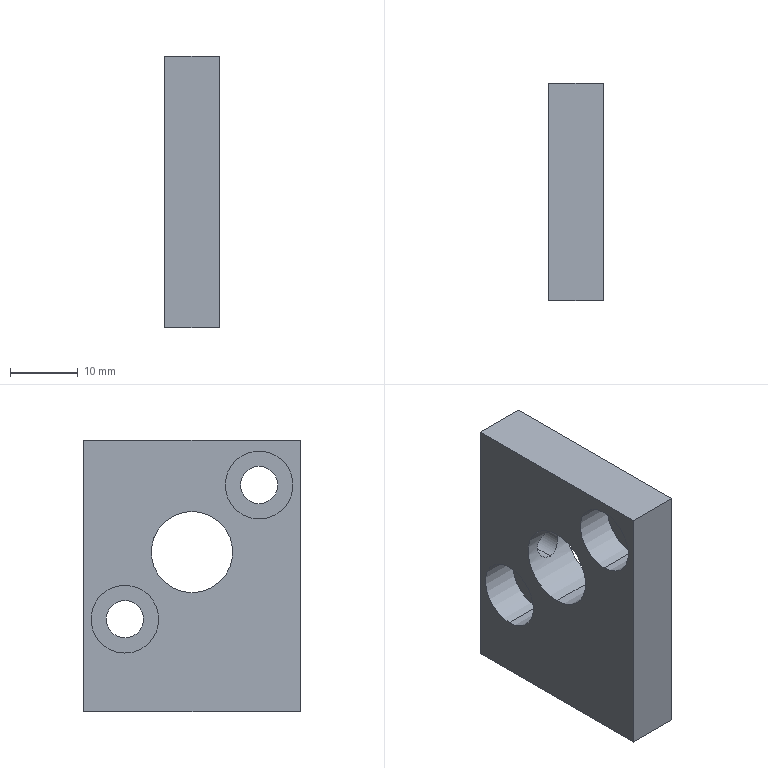Part | SolidWorks | features HoleWzd 2, Extrusion 1, ICE 1 | 1 solid | 28 faces | box 8 x 32 x 40 mm | volume 7835 mm3 | cylinder 16 | plane 8 | cone 4 | commonest cylinder face diameters 4.2 x6 5.5 x4 10 x4 12 x2
STEP:
#1=CARTESIAN_POINT('',(4.,5.396,0.9));
#2=VERTEX_POINT('',#1);
#3=CARTESIAN_POINT('',(4.,5.789,5.1));
#4=VERTEX_POINT('',#3);
#5=CARTESIAN_POINT('',(4.,5.396,0.9));
#6=CARTESIAN_POINT('',(3.724,5.396,0.9));
#7=CARTESIAN_POINT('',(3.445,5.424,0.9562));
#8=CARTESIAN_POINT('',(3.067,5.495,1.114));
#9=CARTESIAN_POINT('',(2.945,5.524,1.179));
#10=CARTESIAN_POINT('',(2.72,5.585,1.33));
#11=CARTESIAN_POINT('',(2.616,5.618,1.415));
#12=CARTESIAN_POINT('',(2.423,5.686,1.606));
#13=CARTESIAN_POINT('',(2.337,5.721,1.71));
#14=CARTESIAN_POINT('',(2.187,5.786,1.932));
#15=CARTESIAN_POINT('',(2.121,5.818,2.052));
#16=CARTESIAN_POINT('',(2.014,5.876,2.303));
#17=CARTESIAN_POINT('',(1.974,5.901,2.432));
#18=CARTESIAN_POINT('',(1.917,5.945,2.699));
#19=CARTESIAN_POINT('',(1.902,5.962,2.839));
#20=CARTESIAN_POINT('',(1.899,5.988,3.115));
#21=CARTESIAN_POINT('',(1.911,5.995,3.252));
#22=CARTESIAN_POINT('',(1.962,6.002,3.525));
#23=CARTESIAN_POINT('',(2.002,6.,3.661));
#24=CARTESIAN_POINT('',(2.158,5.983,4.045));
#25=CARTESIAN_POINT('',(2.314,5.955,4.282));
#26=CARTESIAN_POINT('',(2.604,5.908,4.575));
#27=CARTESIAN_POINT('',(2.712,5.891,4.665));
#28=CARTESIAN_POINT('',(2.941,5.859,4.819));
#29=CARTESIAN_POINT('',(3.062,5.844,4.884));
#30=CARTESIAN_POINT('',(3.318,5.818,4.991));
#31=CARTESIAN_POINT('',(3.452,5.807,5.032));
#32=CARTESIAN_POINT('',(3.722,5.793,5.086));
#33=CARTESIAN_POINT('',(3.86,5.789,5.1));
#34=CARTESIAN_POINT('',(4.,5.789,5.1));
#35=B_SPLINE_CURVE_WITH_KNOTS('',3,(#5,#6,#7,#8,#9,#10,#11,#12,#13,#14,#15,#16,#17,#18,#19,#20,#21,#22,#23,#24,#25,#26,#27,#28,#29,#30,#31,#32,#33,#34),.UNSPECIFIED.,.F.,.F.,(4,2,2,2,2,2,2,2,2,2,2,2,2,2,4),(0.006634,0.007462,0.007877,0.008291,0.008706,0.00912,0.009534,0.009949,0.01036,0.01078,0.01161,0.01202,0.01243,0.01285,0.01326),.UNSPECIFIED.);
#36=EDGE_CURVE('',#2,#4,#35,.T.);
#37=ORIENTED_EDGE('',*,*,#36,.F.);
#38=CARTESIAN_POINT('',(4.,16.,0.9));
#39=VERTEX_POINT('',#38);
#40=CARTESIAN_POINT('',(4.,16.,0.9));
#41=DIRECTION('',(0.,1.,0.));
#42=VECTOR('',#41,1000.);
#43=LINE('',#40,#42);
#44=EDGE_CURVE('',#2,#39,#43,.T.);
#45=ORIENTED_EDGE('',*,*,#44,.T.);
#46=CARTESIAN_POINT('',(4.,16.,5.1));
#47=VERTEX_POINT('',#46);
#48=CARTESIAN_POINT('',(4.,16.,3.));
#49=DIRECTION('',(0.,1.,0.));
#50=DIRECTION('',(0.,0.,1.));
#51=AXIS2_PLACEMENT_3D('',#48,#49,#50);
#52=CIRCLE('',#51,2.1);
#53=EDGE_CURVE('',#39,#47,#52,.T.);
#54=ORIENTED_EDGE('',*,*,#53,.T.);
#55=CARTESIAN_POINT('',(4.,16.,5.1));
#56=DIRECTION('',(0.,1.,0.));
#57=VECTOR('',#56,1000.);
#58=LINE('',#55,#57);
#59=EDGE_CURVE('',#4,#47,#58,.T.);
#60=ORIENTED_EDGE('',*,*,#59,.F.);
#61=EDGE_LOOP('',(#37,#45,#54,#60));
#62=FACE_OUTER_BOUND('',#61,.T.);
#63=CARTESIAN_POINT('',(4.,16.,3.));
#64=DIRECTION('',(0.,1.,0.));
#65=DIRECTION('',(0.,0.,1.));
#66=AXIS2_PLACEMENT_3D('',#63,#64,#65);
#67=CYLINDRICAL_SURFACE('',#66,2.1);
#68=ADVANCED_FACE('',(#62),#67,.F.);
#69=CARTESIAN_POINT('',(4.,3.6,12.9));
#70=VERTEX_POINT('',#69);
#71=CARTESIAN_POINT('',(4.,3.6,17.1));
#72=VERTEX_POINT('',#71);
#73=CARTESIAN_POINT('',(4.,3.6,15.));
#74=DIRECTION('',(0.,1.,0.));
#75=DIRECTION('',(0.,0.,1.));
#76=AXIS2_PLACEMENT_3D('',#73,#74,#75);
#77=CIRCLE('',#76,2.1);
#78=EDGE_CURVE('',#70,#72,#77,.T.);
#79=ORIENTED_EDGE('',*,*,#78,.F.);
#80=CARTESIAN_POINT('',(4.,16.,12.9));
#81=VERTEX_POINT('',#80);
#82=CARTESIAN_POINT('',(4.,16.,12.9));
#83=DIRECTION('',(0.,1.,0.));
#84=VECTOR('',#83,1000.);
#85=LINE('',#82,#84);
#86=EDGE_CURVE('',#70,#81,#85,.T.);
#87=ORIENTED_EDGE('',*,*,#86,.T.);
#88=CARTESIAN_POINT('',(4.,16.,17.1));
#89=VERTEX_POINT('',#88);
#90=CARTESIAN_POINT('',(4.,16.,15.));
#91=DIRECTION('',(0.,1.,0.));
#92=DIRECTION('',(0.,0.,1.));
#93=AXIS2_PLACEMENT_3D('',#90,#91,#92);
#94=CIRCLE('',#93,2.1);
#95=EDGE_CURVE('',#81,#89,#94,.T.);
#96=ORIENTED_EDGE('',*,*,#95,.T.);
#97=CARTESIAN_POINT('',(4.,16.,17.1));
#98=DIRECTION('',(0.,1.,0.));
#99=VECTOR('',#98,1000.);
#100=LINE('',#97,#99);
#101=EDGE_CURVE('',#72,#89,#100,.T.);
#102=ORIENTED_EDGE('',*,*,#101,.F.);
#103=EDGE_LOOP('',(#79,#87,#96,#102));
#104=FACE_OUTER_BOUND('',#103,.T.);
#105=CARTESIAN_POINT('',(4.,16.,15.));
#106=DIRECTION('',(0.,1.,0.));
#107=DIRECTION('',(0.,0.,1.));
#108=AXIS2_PLACEMENT_3D('',#105,#106,#107);
#109=CYLINDRICAL_SURFACE('',#108,2.1);
#110=ADVANCED_FACE('',(#104),#109,.F.);
#111=CARTESIAN_POINT('',(4.,2.338,15.));
#112=VERTEX_POINT('',#111);
#113=CARTESIAN_POINT('',(4.,3.6,17.1));
#114=DIRECTION('',(0.,0.515,0.8572));
#115=VECTOR('',#114,1000.);
#116=LINE('',#113,#115);
#117=EDGE_CURVE('',#112,#72,#116,.T.);
#118=ORIENTED_EDGE('',*,*,#117,.F.);
#119=CARTESIAN_POINT('',(4.,3.6,12.9));
#120=DIRECTION('',(0.,0.515,-0.8572));
#121=VECTOR('',#120,1000.);
#122=LINE('',#119,#121);
#123=EDGE_CURVE('',#112,#70,#122,.T.);
#124=ORIENTED_EDGE('',*,*,#123,.T.);
#125=ORIENTED_EDGE('',*,*,#78,.T.);
#126=EDGE_LOOP('',(#118,#124,#125));
#127=FACE_OUTER_BOUND('',#126,.T.);
#128=CARTESIAN_POINT('',(4.,3.6,15.));
#129=DIRECTION('',(0.,1.,0.));
#130=DIRECTION('',(0.,0.,1.));
#131=AXIS2_PLACEMENT_3D('',#128,#129,#130);
#132=CONICAL_SURFACE('',#131,2.1,1.03);
#133=ADVANCED_FACE('',(#127),#132,.F.);
#134=CARTESIAN_POINT('',(4.,3.6,-17.1));
#135=VERTEX_POINT('',#134);
#136=CARTESIAN_POINT('',(4.,3.6,-12.9));
#137=VERTEX_POINT('',#136);
#138=CARTESIAN_POINT('',(4.,3.6,-15.));
#139=DIRECTION('',(0.,1.,0.));
#140=DIRECTION('',(0.,0.,1.));
#141=AXIS2_PLACEMENT_3D('',#138,#139,#140);
#142=CIRCLE('',#141,2.1);
#143=EDGE_CURVE('',#135,#137,#142,.T.);
#144=ORIENTED_EDGE('',*,*,#143,.F.);
#145=CARTESIAN_POINT('',(4.,16.,-17.1));
#146=VERTEX_POINT('',#145);
#147=CARTESIAN_POINT('',(4.,16.,-17.1));
#148=DIRECTION('',(0.,1.,0.));
#149=VECTOR('',#148,1000.);
#150=LINE('',#147,#149);
#151=EDGE_CURVE('',#135,#146,#150,.T.);
#152=ORIENTED_EDGE('',*,*,#151,.T.);
#153=CARTESIAN_POINT('',(4.,16.,-12.9));
#154=VERTEX_POINT('',#153);
#155=CARTESIAN_POINT('',(4.,16.,-15.));
#156=DIRECTION('',(0.,1.,0.));
#157=DIRECTION('',(0.,0.,1.));
#158=AXIS2_PLACEMENT_3D('',#155,#156,#157);
#159=CIRCLE('',#158,2.1);
#160=EDGE_CURVE('',#146,#154,#159,.T.);
#161=ORIENTED_EDGE('',*,*,#160,.T.);
#162=CARTESIAN_POINT('',(4.,16.,-12.9));
#163=DIRECTION('',(0.,1.,0.));
#164=VECTOR('',#163,1000.);
#165=LINE('',#162,#164);
#166=EDGE_CURVE('',#137,#154,#165,.T.);
#167=ORIENTED_EDGE('',*,*,#166,.F.);
#168=EDGE_LOOP('',(#144,#152,#161,#167));
#169=FACE_OUTER_BOUND('',#168,.T.);
#170=CARTESIAN_POINT('',(4.,16.,-15.));
#171=DIRECTION('',(0.,1.,0.));
#172=DIRECTION('',(0.,0.,1.));
#173=AXIS2_PLACEMENT_3D('',#170,#171,#172);
#174=CYLINDRICAL_SURFACE('',#173,2.1);
#175=ADVANCED_FACE('',(#169),#174,.F.);
#176=CARTESIAN_POINT('',(4.,2.338,-15.));
#177=VERTEX_POINT('',#176);
#178=CARTESIAN_POINT('',(4.,3.6,-12.9));
#179=DIRECTION('',(0.,0.515,0.8572));
#180=VECTOR('',#179,1000.);
#181=LINE('',#178,#180);
#182=EDGE_CURVE('',#177,#137,#181,.T.);
#183=ORIENTED_EDGE('',*,*,#182,.F.);
#184=CARTESIAN_POINT('',(4.,3.6,-17.1));
#185=DIRECTION('',(0.,0.515,-0.8572));
#186=VECTOR('',#185,1000.);
#187=LINE('',#184,#186);
#188=EDGE_CURVE('',#177,#135,#187,.T.);
#189=ORIENTED_EDGE('',*,*,#188,.T.);
#190=ORIENTED_EDGE('',*,*,#143,.T.);
#191=EDGE_LOOP('',(#183,#189,#190));
#192=FACE_OUTER_BOUND('',#191,.T.);
#193=CARTESIAN_POINT('',(4.,3.6,-15.));
#194=DIRECTION('',(0.,1.,0.));
#195=DIRECTION('',(0.,0.,1.));
#196=AXIS2_PLACEMENT_3D('',#193,#194,#195);
#197=CONICAL_SURFACE('',#196,2.1,1.03);
#198=ADVANCED_FACE('',(#192),#197,.F.);
#199=CARTESIAN_POINT('',(5.7,9.899,-11.376));
#200=VERTEX_POINT('',#199);
#201=CARTESIAN_POINT('',(5.7,9.899,-1.376));
#202=VERTEX_POINT('',#201);
#203=CARTESIAN_POINT('',(5.7,9.899,-6.376));
#204=DIRECTION('',(-1.,0.,0.));
#205=DIRECTION('',(0.,0.,1.));
#206=AXIS2_PLACEMENT_3D('',#203,#204,#205);
#207=CIRCLE('',#206,5.);
#208=EDGE_CURVE('',#200,#202,#207,.T.);
#209=ORIENTED_EDGE('',*,*,#208,.F.);
#210=CARTESIAN_POINT('',(0.,9.899,-11.376));
#211=VERTEX_POINT('',#210);
#212=CARTESIAN_POINT('',(0.,9.899,-11.376));
#213=DIRECTION('',(-1.,0.,0.));
#214=VECTOR('',#213,1000.);
#215=LINE('',#212,#214);
#216=EDGE_CURVE('',#200,#211,#215,.T.);
#217=ORIENTED_EDGE('',*,*,#216,.T.);
#218=CARTESIAN_POINT('',(0.,9.899,-1.376));
#219=VERTEX_POINT('',#218);
#220=CARTESIAN_POINT('',(0.,9.899,-6.376));
#221=DIRECTION('',(-1.,0.,0.));
#222=DIRECTION('',(0.,0.,1.));
#223=AXIS2_PLACEMENT_3D('',#220,#221,#222);
#224=CIRCLE('',#223,5.);
#225=EDGE_CURVE('',#211,#219,#224,.T.);
#226=ORIENTED_EDGE('',*,*,#225,.T.);
#227=CARTESIAN_POINT('',(0.,9.899,-1.376));
#228=DIRECTION('',(-1.,0.,0.));
#229=VECTOR('',#228,1000.);
#230=LINE('',#227,#229);
#231=EDGE_CURVE('',#202,#219,#230,.T.);
#232=ORIENTED_EDGE('',*,*,#231,.F.);
#233=EDGE_LOOP('',(#209,#217,#226,#232));
#234=FACE_OUTER_BOUND('',#233,.T.);
#235=CARTESIAN_POINT('',(0.,9.899,-6.376));
#236=DIRECTION('',(-1.,0.,0.));
#237=DIRECTION('',(0.,0.,1.));
#238=AXIS2_PLACEMENT_3D('',#235,#236,#237);
#239=CYLINDRICAL_SURFACE('',#238,5.);
#240=ADVANCED_FACE('',(#234),#239,.F.);
#241=CARTESIAN_POINT('',(8.,9.899,-9.126));
#242=VERTEX_POINT('',#241);
#243=CARTESIAN_POINT('',(8.,9.899,-3.626));
#244=VERTEX_POINT('',#243);
#245=CARTESIAN_POINT('',(8.,9.899,-6.376));
#246=DIRECTION('',(-1.,0.,0.));
#247=DIRECTION('',(0.,0.,1.));
#248=AXIS2_PLACEMENT_3D('',#245,#246,#247);
#249=CIRCLE('',#248,2.75);
#250=EDGE_CURVE('',#242,#244,#249,.T.);
#251=ORIENTED_EDGE('',*,*,#250,.F.);
#252=CARTESIAN_POINT('',(5.7,9.899,-9.126));
#253=VERTEX_POINT('',#252);
#254=CARTESIAN_POINT('',(0.,9.899,-9.126));
#255=DIRECTION('',(-1.,0.,0.));
#256=VECTOR('',#255,1000.);
#257=LINE('',#254,#256);
#258=EDGE_CURVE('',#242,#253,#257,.T.);
#259=ORIENTED_EDGE('',*,*,#258,.T.);
#260=CARTESIAN_POINT('',(5.7,9.899,-3.626));
#261=VERTEX_POINT('',#260);
#262=CARTESIAN_POINT('',(5.7,9.899,-6.376));
#263=DIRECTION('',(-1.,0.,0.));
#264=DIRECTION('',(0.,0.,1.));
#265=AXIS2_PLACEMENT_3D('',#262,#263,#264);
#266=CIRCLE('',#265,2.75);
#267=EDGE_CURVE('',#253,#261,#266,.T.);
#268=ORIENTED_EDGE('',*,*,#267,.T.);
#269=CARTESIAN_POINT('',(0.,9.899,-3.626));
#270=DIRECTION('',(-1.,0.,0.));
#271=VECTOR('',#270,1000.);
#272=LINE('',#269,#271);
#273=EDGE_CURVE('',#244,#261,#272,.T.);
#274=ORIENTED_EDGE('',*,*,#273,.F.);
#275=EDGE_LOOP('',(#251,#259,#268,#274));
#276=FACE_OUTER_BOUND('',#275,.T.);
#277=CARTESIAN_POINT('',(0.,9.899,-6.376));
#278=DIRECTION('',(-1.,0.,0.));
#279=DIRECTION('',(0.,0.,1.));
#280=AXIS2_PLACEMENT_3D('',#277,#278,#279);
#281=CYLINDRICAL_SURFACE('',#280,2.75);
#282=ADVANCED_FACE('',(#276),#281,.F.);
#283=CARTESIAN_POINT('',(5.7,-9.899,8.423));
#284=VERTEX_POINT('',#283);
#285=CARTESIAN_POINT('',(5.7,-9.899,18.423));
#286=VERTEX_POINT('',#285);
#287=CARTESIAN_POINT('',(5.7,-9.899,13.423));
#288=DIRECTION('',(-1.,0.,0.));
#289=DIRECTION('',(0.,0.,1.));
#290=AXIS2_PLACEMENT_3D('',#287,#288,#289);
#291=CIRCLE('',#290,5.);
#292=EDGE_CURVE('',#284,#286,#291,.T.);
#293=ORIENTED_EDGE('',*,*,#292,.F.);
#294=CARTESIAN_POINT('',(0.,-9.899,8.423));
#295=VERTEX_POINT('',#294);
#296=CARTESIAN_POINT('',(0.,-9.899,8.423));
#297=DIRECTION('',(-1.,0.,0.));
#298=VECTOR('',#297,1000.);
#299=LINE('',#296,#298);
#300=EDGE_CURVE('',#284,#295,#299,.T.);
#301=ORIENTED_EDGE('',*,*,#300,.T.);
#302=CARTESIAN_POINT('',(0.,-9.899,18.423));
#303=VERTEX_POINT('',#302);
#304=CARTESIAN_POINT('',(0.,-9.899,13.423));
#305=DIRECTION('',(-1.,0.,0.));
#306=DIRECTION('',(0.,0.,1.));
#307=AXIS2_PLACEMENT_3D('',#304,#305,#306);
#308=CIRCLE('',#307,5.);
#309=EDGE_CURVE('',#295,#303,#308,.T.);
#310=ORIENTED_EDGE('',*,*,#309,.T.);
#311=CARTESIAN_POINT('',(0.,-9.899,18.423));
#312=DIRECTION('',(-1.,0.,0.));
#313=VECTOR('',#312,1000.);
#314=LINE('',#311,#313);
#315=EDGE_CURVE('',#286,#303,#314,.T.);
#316=ORIENTED_EDGE('',*,*,#315,.F.);
#317=EDGE_LOOP('',(#293,#301,#310,#316));
#318=FACE_OUTER_BOUND('',#317,.T.);
#319=CARTESIAN_POINT('',(0.,-9.899,13.423));
#320=DIRECTION('',(-1.,0.,0.));
#321=DIRECTION('',(0.,0.,1.));
#322=AXIS2_PLACEMENT_3D('',#319,#320,#321);
#323=CYLINDRICAL_SURFACE('',#322,5.);
#324=ADVANCED_FACE('',(#318),#323,.F.);
#325=CARTESIAN_POINT('',(8.,-9.899,10.673));
#326=VERTEX_POINT('',#325);
#327=CARTESIAN_POINT('',(8.,-9.899,16.173));
#328=VERTEX_POINT('',#327);
#329=CARTESIAN_POINT('',(8.,-9.899,13.423));
#330=DIRECTION('',(-1.,0.,0.));
#331=DIRECTION('',(0.,0.,1.));
#332=AXIS2_PLACEMENT_3D('',#329,#330,#331);
#333=CIRCLE('',#332,2.75);
#334=EDGE_CURVE('',#326,#328,#333,.T.);
#335=ORIENTED_EDGE('',*,*,#334,.F.);
#336=CARTESIAN_POINT('',(5.7,-9.899,10.673));
#337=VERTEX_POINT('',#336);
#338=CARTESIAN_POINT('',(0.,-9.899,10.673));
#339=DIRECTION('',(-1.,0.,0.));
#340=VECTOR('',#339,1000.);
#341=LINE('',#338,#340);
#342=EDGE_CURVE('',#326,#337,#341,.T.);
#343=ORIENTED_EDGE('',*,*,#342,.T.);
#344=CARTESIAN_POINT('',(5.7,-9.899,16.173));
#345=VERTEX_POINT('',#344);
#346=CARTESIAN_POINT('',(5.7,-9.899,13.423));
#347=DIRECTION('',(-1.,0.,0.));
#348=DIRECTION('',(0.,0.,1.));
#349=AXIS2_PLACEMENT_3D('',#346,#347,#348);
#350=CIRCLE('',#349,2.75);
#351=EDGE_CURVE('',#337,#345,#350,.T.);
#352=ORIENTED_EDGE('',*,*,#351,.T.);
#353=CARTESIAN_POINT('',(0.,-9.899,16.173));
#354=DIRECTION('',(-1.,0.,0.));
#355=VECTOR('',#354,1000.);
#356=LINE('',#353,#355);
#357=EDGE_CURVE('',#328,#345,#356,.T.);
#358=ORIENTED_EDGE('',*,*,#357,.F.);
#359=EDGE_LOOP('',(#335,#343,#352,#358));
#360=FACE_OUTER_BOUND('',#359,.T.);
#361=CARTESIAN_POINT('',(0.,-9.899,13.423));
#362=DIRECTION('',(-1.,0.,0.));
#363=DIRECTION('',(0.,0.,1.));
#364=AXIS2_PLACEMENT_3D('',#361,#362,#363);
#365=CYLINDRICAL_SURFACE('',#364,2.75);
#366=ADVANCED_FACE('',(#360),#365,.F.);
#367=CARTESIAN_POINT('',(8.,0.,-2.476));
#368=VERTEX_POINT('',#367);
#369=CARTESIAN_POINT('',(8.,0.,9.524));
#370=VERTEX_POINT('',#369);
#371=CARTESIAN_POINT('',(8.,0.,3.524));
#372=DIRECTION('',(-1.,0.,0.));
#373=DIRECTION('',(0.,0.,1.));
#374=AXIS2_PLACEMENT_3D('',#371,#372,#373);
#375=CIRCLE('',#374,6.);
#376=EDGE_CURVE('',#368,#370,#375,.T.);
#377=ORIENTED_EDGE('',*,*,#376,.F.);
#378=CARTESIAN_POINT('',(0.,0.,-2.476));
#379=VERTEX_POINT('',#378);
#380=CARTESIAN_POINT('',(8.,0.,-2.476));
#381=DIRECTION('',(-1.,0.,0.));
#382=VECTOR('',#381,1000.);
#383=LINE('',#380,#382);
#384=EDGE_CURVE('',#368,#379,#383,.T.);
#385=ORIENTED_EDGE('',*,*,#384,.T.);
#386=CARTESIAN_POINT('',(0.,0.,9.524));
#387=VERTEX_POINT('',#386);
#388=CARTESIAN_POINT('',(0.,0.,3.524));
#389=DIRECTION('',(-1.,0.,0.));
#390=DIRECTION('',(0.,0.,1.));
#391=AXIS2_PLACEMENT_3D('',#388,#389,#390);
#392=CIRCLE('',#391,6.);
#393=EDGE_CURVE('',#379,#387,#392,.T.);
#394=ORIENTED_EDGE('',*,*,#393,.T.);
#395=CARTESIAN_POINT('',(8.,0.,9.524));
#396=DIRECTION('',(-1.,0.,0.));
#397=VECTOR('',#396,1000.);
#398=LINE('',#395,#397);
#399=EDGE_CURVE('',#370,#387,#398,.T.);
#400=ORIENTED_EDGE('',*,*,#399,.F.);
#401=EDGE_LOOP('',(#377,#385,#394,#400));
#402=FACE_OUTER_BOUND('',#401,.T.);
#403=CARTESIAN_POINT('',(8.,0.,3.524));
#404=DIRECTION('',(-1.,0.,0.));
#405=DIRECTION('',(0.,0.,1.));
#406=AXIS2_PLACEMENT_3D('',#403,#404,#405);
#407=CYLINDRICAL_SURFACE('',#406,6.);
#408=ADVANCED_FACE('',(#402),#407,.F.);
#409=CARTESIAN_POINT('',(0.,16.,20.));
#410=VERTEX_POINT('',#409);
#411=CARTESIAN_POINT('',(0.,-16.,20.));
#412=VERTEX_POINT('',#411);
#413=CARTESIAN_POINT('',(0.,16.,20.));
#414=DIRECTION('',(0.,-1.,0.));
#415=VECTOR('',#414,1000.);
#416=LINE('',#413,#415);
#417=EDGE_CURVE('',#410,#412,#416,.T.);
#418=ORIENTED_EDGE('',*,*,#417,.T.);
#419=CARTESIAN_POINT('',(8.,-16.,20.));
#420=VERTEX_POINT('',#419);
#421=CARTESIAN_POINT('',(8.,-16.,20.));
#422=DIRECTION('',(-1.,0.,0.));
#423=VECTOR('',#422,1000.);
#424=LINE('',#421,#423);
#425=EDGE_CURVE('',#420,#412,#424,.T.);
#426=ORIENTED_EDGE('',*,*,#425,.F.);
#427=CARTESIAN_POINT('',(8.,16.,20.));
#428=VERTEX_POINT('',#427);
#429=CARTESIAN_POINT('',(8.,16.,20.));
#430=DIRECTION('',(0.,-1.,0.));
#431=VECTOR('',#430,1000.);
#432=LINE('',#429,#431);
#433=EDGE_CURVE('',#428,#420,#432,.T.);
#434=ORIENTED_EDGE('',*,*,#433,.F.);
#435=CARTESIAN_POINT('',(8.,16.,20.));
#436=DIRECTION('',(-1.,0.,0.));
#437=VECTOR('',#436,1000.);
#438=LINE('',#435,#437);
#439=EDGE_CURVE('',#428,#410,#438,.T.);
#440=ORIENTED_EDGE('',*,*,#439,.T.);
#441=EDGE_LOOP('',(#418,#426,#434,#440));
#442=FACE_OUTER_BOUND('',#441,.T.);
#443=CARTESIAN_POINT('',(8.,16.,20.));
#444=DIRECTION('',(0.,0.,-1.));
#445=DIRECTION('',(0.,1.,0.));
#446=AXIS2_PLACEMENT_3D('',#443,#444,#445);
#447=PLANE('',#446);
#448=ADVANCED_FACE('',(#442),#447,.F.);
#449=CARTESIAN_POINT('',(0.,-16.,-20.));
#450=VERTEX_POINT('',#449);
#451=CARTESIAN_POINT('',(0.,-16.,-20.));
#452=DIRECTION('',(0.,0.,-1.));
#453=VECTOR('',#452,1000.);
#454=LINE('',#451,#453);
#455=EDGE_CURVE('',#412,#450,#454,.T.);
#456=ORIENTED_EDGE('',*,*,#455,.T.);
#457=CARTESIAN_POINT('',(8.,-16.,-20.));
#458=VERTEX_POINT('',#457);
#459=CARTESIAN_POINT('',(8.,-16.,-20.));
#460=DIRECTION('',(-1.,0.,0.));
#461=VECTOR('',#460,1000.);
#462=LINE('',#459,#461);
#463=EDGE_CURVE('',#458,#450,#462,.T.);
#464=ORIENTED_EDGE('',*,*,#463,.F.);
#465=CARTESIAN_POINT('',(8.,-16.,-20.));
#466=DIRECTION('',(0.,0.,-1.));
#467=VECTOR('',#466,1000.);
#468=LINE('',#465,#467);
#469=EDGE_CURVE('',#420,#458,#468,.T.);
#470=ORIENTED_EDGE('',*,*,#469,.F.);
#471=ORIENTED_EDGE('',*,*,#425,.T.);
#472=EDGE_LOOP('',(#456,#464,#470,#471));
#473=FACE_OUTER_BOUND('',#472,.T.);
#474=CARTESIAN_POINT('',(8.,-16.,-20.));
#475=DIRECTION('',(0.,1.,0.));
#476=DIRECTION('',(0.,0.,1.));
#477=AXIS2_PLACEMENT_3D('',#474,#475,#476);
#478=PLANE('',#477);
#479=ADVANCED_FACE('',(#473),#478,.F.);
#480=CARTESIAN_POINT('',(0.,16.,-20.));
#481=VERTEX_POINT('',#480);
#482=CARTESIAN_POINT('',(0.,16.,-20.));
#483=DIRECTION('',(0.,1.,0.));
#484=VECTOR('',#483,1000.);
#485=LINE('',#482,#484);
#486=EDGE_CURVE('',#450,#481,#485,.T.);
#487=ORIENTED_EDGE('',*,*,#486,.T.);
#488=CARTESIAN_POINT('',(8.,16.,-20.));
#489=VERTEX_POINT('',#488);
#490=CARTESIAN_POINT('',(8.,16.,-20.));
#491=DIRECTION('',(-1.,0.,0.));
#492=VECTOR('',#491,1000.);
#493=LINE('',#490,#492);
#494=EDGE_CURVE('',#489,#481,#493,.T.);
#495=ORIENTED_EDGE('',*,*,#494,.F.);
#496=CARTESIAN_POINT('',(8.,16.,-20.));
#497=DIRECTION('',(0.,1.,0.));
#498=VECTOR('',#497,1000.);
#499=LINE('',#496,#498);
#500=EDGE_CURVE('',#458,#489,#499,.T.);
#501=ORIENTED_EDGE('',*,*,#500,.F.);
#502=ORIENTED_EDGE('',*,*,#463,.T.);
#503=EDGE_LOOP('',(#487,#495,#501,#502));
#504=FACE_OUTER_BOUND('',#503,.T.);
#505=CARTESIAN_POINT('',(8.,16.,-20.));
#506=DIRECTION('',(0.,0.,1.));
#507=DIRECTION('',(0.,-1.,0.));
#508=AXIS2_PLACEMENT_3D('',#505,#506,#507);
#509=PLANE('',#508);
#510=ADVANCED_FACE('',(#504),#509,.F.);
#511=CARTESIAN_POINT('',(4.,16.,3.));
#512=DIRECTION('',(0.,1.,0.));
#513=DIRECTION('',(0.,0.,1.));
#514=AXIS2_PLACEMENT_3D('',#511,#512,#513);
#515=CIRCLE('',#514,2.1);
#516=EDGE_CURVE('',#47,#39,#515,.T.);
#517=ORIENTED_EDGE('',*,*,#516,.F.);
#518=ORIENTED_EDGE('',*,*,#53,.F.);
#519=EDGE_LOOP('',(#517,#518));
#520=FACE_BOUND('',#519,.T.);
#521=CARTESIAN_POINT('',(4.,16.,15.));
#522=DIRECTION('',(0.,1.,0.));
#523=DIRECTION('',(0.,0.,1.));
#524=AXIS2_PLACEMENT_3D('',#521,#522,#523);
#525=CIRCLE('',#524,2.1);
#526=EDGE_CURVE('',#89,#81,#525,.T.);
#527=ORIENTED_EDGE('',*,*,#526,.F.);
#528=ORIENTED_EDGE('',*,*,#95,.F.);
#529=EDGE_LOOP('',(#527,#528));
#530=FACE_BOUND('',#529,.T.);
#531=CARTESIAN_POINT('',(4.,16.,-15.));
#532=DIRECTION('',(0.,1.,0.));
#533=DIRECTION('',(0.,0.,1.));
#534=AXIS2_PLACEMENT_3D('',#531,#532,#533);
#535=CIRCLE('',#534,2.1);
#536=EDGE_CURVE('',#154,#146,#535,.T.);
#537=ORIENTED_EDGE('',*,*,#536,.F.);
#538=ORIENTED_EDGE('',*,*,#160,.F.);
#539=EDGE_LOOP('',(#537,#538));
#540=FACE_BOUND('',#539,.T.);
#541=CARTESIAN_POINT('',(0.,16.,-20.));
#542=DIRECTION('',(0.,0.,1.));
#543=VECTOR('',#542,1000.);
#544=LINE('',#541,#543);
#545=EDGE_CURVE('',#481,#410,#544,.T.);
#546=ORIENTED_EDGE('',*,*,#545,.T.);
#547=ORIENTED_EDGE('',*,*,#439,.F.);
#548=CARTESIAN_POINT('',(8.,16.,-20.));
#549=DIRECTION('',(0.,0.,1.));
#550=VECTOR('',#549,1000.);
#551=LINE('',#548,#550);
#552=EDGE_CURVE('',#489,#428,#551,.T.);
#553=ORIENTED_EDGE('',*,*,#552,.F.);
#554=ORIENTED_EDGE('',*,*,#494,.T.);
#555=EDGE_LOOP('',(#546,#547,#553,#554));
#556=FACE_OUTER_BOUND('',#555,.T.);
#557=CARTESIAN_POINT('',(8.,16.,-20.));
#558=DIRECTION('',(0.,-1.,0.));
#559=DIRECTION('',(0.,0.,-1.));
#560=AXIS2_PLACEMENT_3D('',#557,#558,#559);
#561=PLANE('',#560);
#562=ADVANCED_FACE('',(#520,#530,#540,#556),#561,.F.);
#563=CARTESIAN_POINT('',(8.,9.899,-6.376));
#564=DIRECTION('',(-1.,0.,0.));
#565=DIRECTION('',(0.,0.,1.));
#566=AXIS2_PLACEMENT_3D('',#563,#564,#565);
#567=CIRCLE('',#566,2.75);
#568=EDGE_CURVE('',#244,#242,#567,.T.);
#569=ORIENTED_EDGE('',*,*,#568,.T.);
#570=ORIENTED_EDGE('',*,*,#250,.T.);
#571=EDGE_LOOP('',(#569,#570));
#572=FACE_BOUND('',#571,.T.);
#573=CARTESIAN_POINT('',(8.,-9.899,13.423));
#574=DIRECTION('',(-1.,0.,0.));
#575=DIRECTION('',(0.,0.,1.));
#576=AXIS2_PLACEMENT_3D('',#573,#574,#575);
#577=CIRCLE('',#576,2.75);
#578=EDGE_CURVE('',#328,#326,#577,.T.);
#579=ORIENTED_EDGE('',*,*,#578,.T.);
#580=ORIENTED_EDGE('',*,*,#334,.T.);
#581=EDGE_LOOP('',(#579,#580));
#582=FACE_BOUND('',#581,.T.);
#583=CARTESIAN_POINT('',(8.,0.,3.524));
#584=DIRECTION('',(-1.,0.,0.));
#585=DIRECTION('',(0.,0.,1.));
#586=AXIS2_PLACEMENT_3D('',#583,#584,#585);
#587=CIRCLE('',#586,6.);
#588=EDGE_CURVE('',#370,#368,#587,.T.);
#589=ORIENTED_EDGE('',*,*,#588,.T.);
#590=ORIENTED_EDGE('',*,*,#376,.T.);
#591=EDGE_LOOP('',(#589,#590));
#592=FACE_BOUND('',#591,.T.);
#593=ORIENTED_EDGE('',*,*,#433,.T.);
#594=ORIENTED_EDGE('',*,*,#469,.T.);
#595=ORIENTED_EDGE('',*,*,#500,.T.);
#596=ORIENTED_EDGE('',*,*,#552,.T.);
#597=EDGE_LOOP('',(#593,#594,#595,#596));
#598=FACE_OUTER_BOUND('',#597,.T.);
#599=CARTESIAN_POINT('',(8.,0.,0.));
#600=DIRECTION('',(-1.,0.,0.));
#601=DIRECTION('',(0.,0.,1.));
#602=AXIS2_PLACEMENT_3D('',#599,#600,#601);
#603=PLANE('',#602);
#604=ADVANCED_FACE('',(#572,#582,#592,#598),#603,.F.);
#605=CARTESIAN_POINT('',(0.,9.899,-6.376));
#606=DIRECTION('',(-1.,0.,0.));
#607=DIRECTION('',(0.,0.,1.));
#608=AXIS2_PLACEMENT_3D('',#605,#606,#607);
#609=CIRCLE('',#608,5.);
#610=EDGE_CURVE('',#219,#211,#609,.T.);
#611=ORIENTED_EDGE('',*,*,#610,.F.);
#612=ORIENTED_EDGE('',*,*,#225,.F.);
#613=EDGE_LOOP('',(#611,#612));
#614=FACE_BOUND('',#613,.T.);
#615=CARTESIAN_POINT('',(0.,-9.899,13.423));
#616=DIRECTION('',(-1.,0.,0.));
#617=DIRECTION('',(0.,0.,1.));
#618=AXIS2_PLACEMENT_3D('',#615,#616,#617);
#619=CIRCLE('',#618,5.);
#620=EDGE_CURVE('',#303,#295,#619,.T.);
#621=ORIENTED_EDGE('',*,*,#620,.F.);
#622=ORIENTED_EDGE('',*,*,#309,.F.);
#623=EDGE_LOOP('',(#621,#622));
#624=FACE_BOUND('',#623,.T.);
#625=CARTESIAN_POINT('',(0.,0.,3.524));
#626=DIRECTION('',(-1.,0.,0.));
#627=DIRECTION('',(0.,0.,1.));
#628=AXIS2_PLACEMENT_3D('',#625,#626,#627);
#629=CIRCLE('',#628,6.);
#630=EDGE_CURVE('',#387,#379,#629,.T.);
#631=ORIENTED_EDGE('',*,*,#630,.F.);
#632=ORIENTED_EDGE('',*,*,#393,.F.);
#633=EDGE_LOOP('',(#631,#632));
#634=FACE_BOUND('',#633,.T.);
#635=ORIENTED_EDGE('',*,*,#417,.F.);
#636=ORIENTED_EDGE('',*,*,#545,.F.);
#637=ORIENTED_EDGE('',*,*,#486,.F.);
#638=ORIENTED_EDGE('',*,*,#455,.F.);
#639=EDGE_LOOP('',(#635,#636,#637,#638));
#640=FACE_OUTER_BOUND('',#639,.T.);
#641=CARTESIAN_POINT('',(0.,0.,0.));
#642=DIRECTION('',(-1.,0.,0.));
#643=DIRECTION('',(0.,0.,1.));
#644=AXIS2_PLACEMENT_3D('',#641,#642,#643);
#645=PLANE('',#644);
#646=ADVANCED_FACE('',(#614,#624,#634,#640),#645,.T.);
#647=ORIENTED_EDGE('',*,*,#384,.F.);
#648=ORIENTED_EDGE('',*,*,#588,.F.);
#649=ORIENTED_EDGE('',*,*,#399,.T.);
#650=ORIENTED_EDGE('',*,*,#630,.T.);
#651=EDGE_LOOP('',(#647,#648,#649,#650));
#652=FACE_OUTER_BOUND('',#651,.T.);
#653=CARTESIAN_POINT('',(4.,5.789,5.1));
#654=CARTESIAN_POINT('',(4.14,5.789,5.1));
#655=CARTESIAN_POINT('',(4.278,5.793,5.086));
#656=CARTESIAN_POINT('',(4.549,5.807,5.032));
#657=CARTESIAN_POINT('',(4.683,5.818,4.991));
#658=CARTESIAN_POINT('',(4.939,5.844,4.884));
#659=CARTESIAN_POINT('',(5.06,5.859,4.818));
#660=CARTESIAN_POINT('',(5.288,5.891,4.664));
#661=CARTESIAN_POINT('',(5.396,5.908,4.575));
#662=CARTESIAN_POINT('',(5.686,5.955,4.282));
#663=CARTESIAN_POINT('',(5.842,5.983,4.045));
#664=CARTESIAN_POINT('',(5.998,6.,3.661));
#665=CARTESIAN_POINT('',(6.038,6.002,3.526));
#666=CARTESIAN_POINT('',(6.089,5.995,3.253));
#667=CARTESIAN_POINT('',(6.101,5.988,3.115));
#668=CARTESIAN_POINT('',(6.098,5.962,2.839));
#669=CARTESIAN_POINT('',(6.083,5.945,2.699));
#670=CARTESIAN_POINT('',(6.026,5.901,2.432));
#671=CARTESIAN_POINT('',(5.985,5.876,2.302));
#672=CARTESIAN_POINT('',(5.878,5.818,2.05));
#673=CARTESIAN_POINT('',(5.813,5.786,1.931));
#674=CARTESIAN_POINT('',(5.662,5.72,1.709));
#675=CARTESIAN_POINT('',(5.574,5.685,1.604));
#676=CARTESIAN_POINT('',(5.383,5.618,1.414));
#677=CARTESIAN_POINT('',(5.279,5.585,1.329));
#678=CARTESIAN_POINT('',(5.054,5.523,1.179));
#679=CARTESIAN_POINT('',(4.932,5.495,1.113));
#680=CARTESIAN_POINT('',(4.68,5.448,1.009));
#681=CARTESIAN_POINT('',(4.55,5.429,0.9685));
#682=CARTESIAN_POINT('',(4.278,5.403,0.9139));
#683=CARTESIAN_POINT('',(4.138,5.396,0.9));
#684=CARTESIAN_POINT('',(4.,5.396,0.9));
#685=B_SPLINE_CURVE_WITH_KNOTS('',3,(#653,#654,#655,#656,#657,#658,#659,#660,#661,#662,#663,#664,#665,#666,#667,#668,#669,#670,#671,#672,#673,#674,#675,#676,#677,#678,#679,#680,#681,#682,#683,#684),.UNSPECIFIED.,.F.,.F.,(4,2,2,2,2,2,2,2,2,2,2,2,2,2,2,4),(0.,0.0004146,0.0008292,0.001244,0.001658,0.002488,0.002902,0.003317,0.003732,0.004146,0.004561,0.004975,0.00539,0.005805,0.006219,0.006634),.UNSPECIFIED.);
#686=EDGE_CURVE('',#4,#2,#685,.T.);
#687=ORIENTED_EDGE('',*,*,#686,.T.);
#688=ORIENTED_EDGE('',*,*,#36,.T.);
#689=EDGE_LOOP('',(#687,#688));
#690=FACE_BOUND('',#689,.T.);
#691=CARTESIAN_POINT('',(8.,0.,3.524));
#692=DIRECTION('',(-1.,0.,0.));
#693=DIRECTION('',(0.,0.,1.));
#694=AXIS2_PLACEMENT_3D('',#691,#692,#693);
#695=CYLINDRICAL_SURFACE('',#694,6.);
#696=ADVANCED_FACE('',(#652,#690),#695,.F.);
#697=ORIENTED_EDGE('',*,*,#342,.F.);
#698=ORIENTED_EDGE('',*,*,#578,.F.);
#699=ORIENTED_EDGE('',*,*,#357,.T.);
#700=CARTESIAN_POINT('',(5.7,-9.899,13.423));
#701=DIRECTION('',(-1.,0.,0.));
#702=DIRECTION('',(0.,0.,1.));
#703=AXIS2_PLACEMENT_3D('',#700,#701,#702);
#704=CIRCLE('',#703,2.75);
#705=EDGE_CURVE('',#345,#337,#704,.T.);
#706=ORIENTED_EDGE('',*,*,#705,.T.);
#707=EDGE_LOOP('',(#697,#698,#699,#706));
#708=FACE_OUTER_BOUND('',#707,.T.);
#709=CARTESIAN_POINT('',(0.,-9.899,13.423));
#710=DIRECTION('',(-1.,0.,0.));
#711=DIRECTION('',(0.,0.,1.));
#712=AXIS2_PLACEMENT_3D('',#709,#710,#711);
#713=CYLINDRICAL_SURFACE('',#712,2.75);
#714=ADVANCED_FACE('',(#708),#713,.F.);
#715=ORIENTED_EDGE('',*,*,#705,.F.);
#716=ORIENTED_EDGE('',*,*,#351,.F.);
#717=EDGE_LOOP('',(#715,#716));
#718=FACE_BOUND('',#717,.T.);
#719=CARTESIAN_POINT('',(5.7,-9.899,13.423));
#720=DIRECTION('',(-1.,0.,0.));
#721=DIRECTION('',(0.,0.,1.));
#722=AXIS2_PLACEMENT_3D('',#719,#720,#721);
#723=CIRCLE('',#722,5.);
#724=EDGE_CURVE('',#286,#284,#723,.T.);
#725=ORIENTED_EDGE('',*,*,#724,.T.);
#726=ORIENTED_EDGE('',*,*,#292,.T.);
#727=EDGE_LOOP('',(#725,#726));
#728=FACE_OUTER_BOUND('',#727,.T.);
#729=CARTESIAN_POINT('',(5.7,-7.149,13.423));
#730=DIRECTION('',(1.,0.,0.));
#731=DIRECTION('',(0.,0.,-1.));
#732=AXIS2_PLACEMENT_3D('',#729,#730,#731);
#733=PLANE('',#732);
#734=ADVANCED_FACE('',(#718,#728),#733,.F.);
#735=ORIENTED_EDGE('',*,*,#300,.F.);
#736=ORIENTED_EDGE('',*,*,#724,.F.);
#737=ORIENTED_EDGE('',*,*,#315,.T.);
#738=ORIENTED_EDGE('',*,*,#620,.T.);
#739=EDGE_LOOP('',(#735,#736,#737,#738));
#740=FACE_OUTER_BOUND('',#739,.T.);
#741=CARTESIAN_POINT('',(0.,-9.899,13.423));
#742=DIRECTION('',(-1.,0.,0.));
#743=DIRECTION('',(0.,0.,1.));
#744=AXIS2_PLACEMENT_3D('',#741,#742,#743);
#745=CYLINDRICAL_SURFACE('',#744,5.);
#746=ADVANCED_FACE('',(#740),#745,.F.);
#747=ORIENTED_EDGE('',*,*,#258,.F.);
#748=ORIENTED_EDGE('',*,*,#568,.F.);
#749=ORIENTED_EDGE('',*,*,#273,.T.);
#750=CARTESIAN_POINT('',(5.7,9.899,-6.376));
#751=DIRECTION('',(-1.,0.,0.));
#752=DIRECTION('',(0.,0.,1.));
#753=AXIS2_PLACEMENT_3D('',#750,#751,#752);
#754=CIRCLE('',#753,2.75);
#755=EDGE_CURVE('',#261,#253,#754,.T.);
#756=ORIENTED_EDGE('',*,*,#755,.T.);
#757=EDGE_LOOP('',(#747,#748,#749,#756));
#758=FACE_OUTER_BOUND('',#757,.T.);
#759=CARTESIAN_POINT('',(0.,9.899,-6.376));
#760=DIRECTION('',(-1.,0.,0.));
#761=DIRECTION('',(0.,0.,1.));
#762=AXIS2_PLACEMENT_3D('',#759,#760,#761);
#763=CYLINDRICAL_SURFACE('',#762,2.75);
#764=ADVANCED_FACE('',(#758),#763,.F.);
#765=ORIENTED_EDGE('',*,*,#755,.F.);
#766=ORIENTED_EDGE('',*,*,#267,.F.);
#767=EDGE_LOOP('',(#765,#766));
#768=FACE_BOUND('',#767,.T.);
#769=CARTESIAN_POINT('',(5.7,9.899,-6.376));
#770=DIRECTION('',(-1.,0.,0.));
#771=DIRECTION('',(0.,0.,1.));
#772=AXIS2_PLACEMENT_3D('',#769,#770,#771);
#773=CIRCLE('',#772,5.);
#774=EDGE_CURVE('',#202,#200,#773,.T.);
#775=ORIENTED_EDGE('',*,*,#774,.T.);
#776=ORIENTED_EDGE('',*,*,#208,.T.);
#777=EDGE_LOOP('',(#775,#776));
#778=FACE_OUTER_BOUND('',#777,.T.);
#779=CARTESIAN_POINT('',(5.7,12.649,-6.376));
#780=DIRECTION('',(1.,0.,0.));
#781=DIRECTION('',(0.,0.,-1.));
#782=AXIS2_PLACEMENT_3D('',#779,#780,#781);
#783=PLANE('',#782);
#784=ADVANCED_FACE('',(#768,#778),#783,.F.);
#785=ORIENTED_EDGE('',*,*,#216,.F.);
#786=ORIENTED_EDGE('',*,*,#774,.F.);
#787=ORIENTED_EDGE('',*,*,#231,.T.);
#788=ORIENTED_EDGE('',*,*,#610,.T.);
#789=EDGE_LOOP('',(#785,#786,#787,#788));
#790=FACE_OUTER_BOUND('',#789,.T.);
#791=CARTESIAN_POINT('',(0.,9.899,-6.376));
#792=DIRECTION('',(-1.,0.,0.));
#793=DIRECTION('',(0.,0.,1.));
#794=AXIS2_PLACEMENT_3D('',#791,#792,#793);
#795=CYLINDRICAL_SURFACE('',#794,5.);
#796=ADVANCED_FACE('',(#790),#795,.F.);
#797=ORIENTED_EDGE('',*,*,#188,.F.);
#798=ORIENTED_EDGE('',*,*,#182,.T.);
#799=CARTESIAN_POINT('',(4.,3.6,-15.));
#800=DIRECTION('',(0.,1.,0.));
#801=DIRECTION('',(0.,0.,1.));
#802=AXIS2_PLACEMENT_3D('',#799,#800,#801);
#803=CIRCLE('',#802,2.1);
#804=EDGE_CURVE('',#137,#135,#803,.T.);
#805=ORIENTED_EDGE('',*,*,#804,.T.);
#806=EDGE_LOOP('',(#797,#798,#805));
#807=FACE_OUTER_BOUND('',#806,.T.);
#808=CARTESIAN_POINT('',(4.,3.6,-15.));
#809=DIRECTION('',(0.,1.,0.));
#810=DIRECTION('',(0.,0.,1.));
#811=AXIS2_PLACEMENT_3D('',#808,#809,#810);
#812=CONICAL_SURFACE('',#811,2.1,1.03);
#813=ADVANCED_FACE('',(#807),#812,.F.);
#814=ORIENTED_EDGE('',*,*,#151,.F.);
#815=ORIENTED_EDGE('',*,*,#804,.F.);
#816=ORIENTED_EDGE('',*,*,#166,.T.);
#817=ORIENTED_EDGE('',*,*,#536,.T.);
#818=EDGE_LOOP('',(#814,#815,#816,#817));
#819=FACE_OUTER_BOUND('',#818,.T.);
#820=CARTESIAN_POINT('',(4.,16.,-15.));
#821=DIRECTION('',(0.,1.,0.));
#822=DIRECTION('',(0.,0.,1.));
#823=AXIS2_PLACEMENT_3D('',#820,#821,#822);
#824=CYLINDRICAL_SURFACE('',#823,2.1);
#825=ADVANCED_FACE('',(#819),#824,.F.);
#826=ORIENTED_EDGE('',*,*,#123,.F.);
#827=ORIENTED_EDGE('',*,*,#117,.T.);
#828=CARTESIAN_POINT('',(4.,3.6,15.));
#829=DIRECTION('',(0.,1.,0.));
#830=DIRECTION('',(0.,0.,1.));
#831=AXIS2_PLACEMENT_3D('',#828,#829,#830);
#832=CIRCLE('',#831,2.1);
#833=EDGE_CURVE('',#72,#70,#832,.T.);
#834=ORIENTED_EDGE('',*,*,#833,.T.);
#835=EDGE_LOOP('',(#826,#827,#834));
#836=FACE_OUTER_BOUND('',#835,.T.);
#837=CARTESIAN_POINT('',(4.,3.6,15.));
#838=DIRECTION('',(0.,1.,0.));
#839=DIRECTION('',(0.,0.,1.));
#840=AXIS2_PLACEMENT_3D('',#837,#838,#839);
#841=CONICAL_SURFACE('',#840,2.1,1.03);
#842=ADVANCED_FACE('',(#836),#841,.F.);
#843=ORIENTED_EDGE('',*,*,#86,.F.);
#844=ORIENTED_EDGE('',*,*,#833,.F.);
#845=ORIENTED_EDGE('',*,*,#101,.T.);
#846=ORIENTED_EDGE('',*,*,#526,.T.);
#847=EDGE_LOOP('',(#843,#844,#845,#846));
#848=FACE_OUTER_BOUND('',#847,.T.);
#849=CARTESIAN_POINT('',(4.,16.,15.));
#850=DIRECTION('',(0.,1.,0.));
#851=DIRECTION('',(0.,0.,1.));
#852=AXIS2_PLACEMENT_3D('',#849,#850,#851);
#853=CYLINDRICAL_SURFACE('',#852,2.1);
#854=ADVANCED_FACE('',(#848),#853,.F.);
#855=ORIENTED_EDGE('',*,*,#44,.F.);
#856=ORIENTED_EDGE('',*,*,#686,.F.);
#857=ORIENTED_EDGE('',*,*,#59,.T.);
#858=ORIENTED_EDGE('',*,*,#516,.T.);
#859=EDGE_LOOP('',(#855,#856,#857,#858));
#860=FACE_OUTER_BOUND('',#859,.T.);
#861=CARTESIAN_POINT('',(4.,16.,3.));
#862=DIRECTION('',(0.,1.,0.));
#863=DIRECTION('',(0.,0.,1.));
#864=AXIS2_PLACEMENT_3D('',#861,#862,#863);
#865=CYLINDRICAL_SURFACE('',#864,2.1);
#866=ADVANCED_FACE('',(#860),#865,.F.);
#867=CLOSED_SHELL('',(#68,#110,#133,#175,#198,#240,#282,#324,#366,#408,#448,#479,#510,#562,#604,#646,#696,#714,#734,#746,#764,#784,#796,#813,#825,#842,#854,#866));
#868=MANIFOLD_SOLID_BREP('',#867);
#869=CARTESIAN_POINT('',(0.,0.,0.));
#870=DIRECTION('',(0.,0.,1.));
#871=DIRECTION('',(1.,0.,0.));
#872=AXIS2_PLACEMENT_3D('',#869,#870,#871);
#873=(LENGTH_UNIT()NAMED_UNIT(*)SI_UNIT(.MILLI.,.METRE.));
#874=UNCERTAINTY_MEASURE_WITH_UNIT(LENGTH_MEASURE(0.00001),#873,'','');
#875=(NAMED_UNIT(*)PLANE_ANGLE_UNIT()SI_UNIT($,.RADIAN.));
#876=(NAMED_UNIT(*)SI_UNIT($,.STERADIAN.)SOLID_ANGLE_UNIT());
#877=(GEOMETRIC_REPRESENTATION_CONTEXT(3)GLOBAL_UNCERTAINTY_ASSIGNED_CONTEXT((#874))GLOBAL_UNIT_ASSIGNED_CONTEXT((#873,#875,#876))REPRESENTATION_CONTEXT('',''));
#878=ADVANCED_BREP_SHAPE_REPRESENTATION('',(#868,#872),#877);